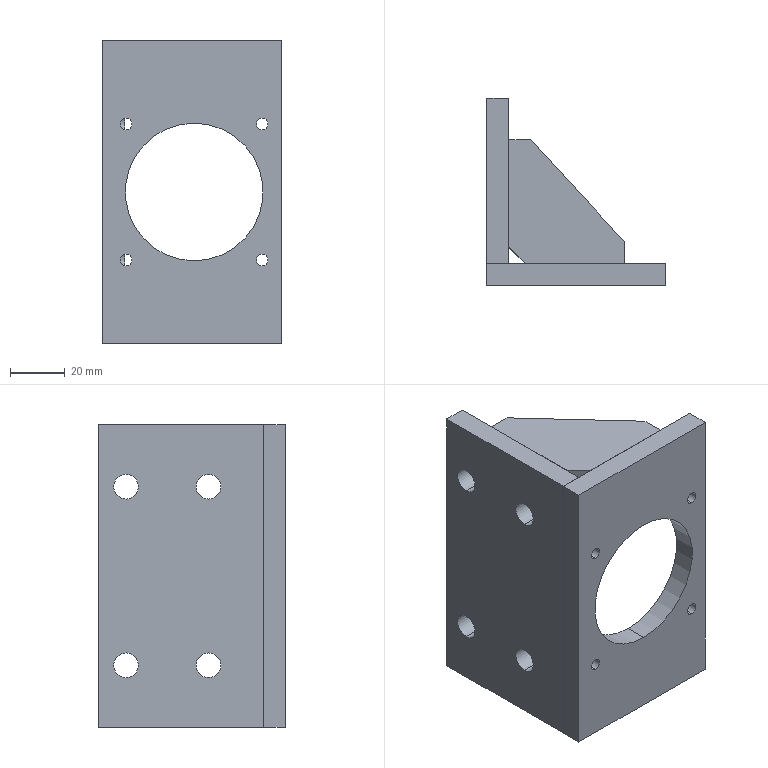Part | STEP file | Motor bracket | 4 solids | 50 faces | box 65 x 68 x 110 mm | volume 111617 mm3 | plane 28 | cylinder 20 | cone 2 | commonest cylinder face diameters 4.2 x10 9 x8 50.1 x2
STEP:
#1=CARTESIAN_POINT('',(-24.5,53.,55.));
#2=VERTEX_POINT('',#1);
#3=CARTESIAN_POINT('',(-24.5,14.,55.));
#4=VERTEX_POINT('',#3);
#5=CARTESIAN_POINT('',(-24.5,14.,55.));
#6=DIRECTION('',(0.,-1.,0.));
#7=VECTOR('',#6,1000.);
#8=LINE('',#5,#7);
#9=EDGE_CURVE('',#2,#4,#8,.T.);
#10=ORIENTED_EDGE('',*,*,#9,.F.);
#11=CARTESIAN_POINT('',(-24.5,53.,47.));
#12=VERTEX_POINT('',#11);
#13=CARTESIAN_POINT('',(-24.5,53.,47.));
#14=DIRECTION('',(0.,0.,1.));
#15=VECTOR('',#14,1000.);
#16=LINE('',#13,#15);
#17=EDGE_CURVE('',#12,#2,#16,.T.);
#18=ORIENTED_EDGE('',*,*,#17,.F.);
#19=CARTESIAN_POINT('',(-24.5,14.,47.));
#20=VERTEX_POINT('',#19);
#21=CARTESIAN_POINT('',(-24.5,14.,47.));
#22=DIRECTION('',(0.,-1.,0.));
#23=VECTOR('',#22,1000.);
#24=LINE('',#21,#23);
#25=EDGE_CURVE('',#12,#20,#24,.T.);
#26=ORIENTED_EDGE('',*,*,#25,.T.);
#27=CARTESIAN_POINT('',(-24.5,14.,47.));
#28=DIRECTION('',(0.,0.,1.));
#29=VECTOR('',#28,1000.);
#30=LINE('',#27,#29);
#31=EDGE_CURVE('',#20,#4,#30,.T.);
#32=ORIENTED_EDGE('',*,*,#31,.T.);
#33=EDGE_LOOP('',(#10,#18,#26,#32));
#34=FACE_OUTER_BOUND('',#33,.T.);
#35=CARTESIAN_POINT('',(-24.5,14.,47.));
#36=DIRECTION('',(-1.,0.,0.));
#37=DIRECTION('',(0.,0.,1.));
#38=AXIS2_PLACEMENT_3D('',#35,#36,#37);
#39=PLANE('',#38);
#40=ADVANCED_FACE('',(#34),#39,.T.);
#41=CARTESIAN_POINT('',(-16.5,53.,55.));
#42=VERTEX_POINT('',#41);
#43=CARTESIAN_POINT('',(-24.5,53.,55.));
#44=DIRECTION('',(-1.,0.,0.));
#45=VECTOR('',#44,1000.);
#46=LINE('',#43,#45);
#47=EDGE_CURVE('',#42,#2,#46,.T.);
#48=ORIENTED_EDGE('',*,*,#47,.F.);
#49=CARTESIAN_POINT('',(-16.5,53.,47.));
#50=VERTEX_POINT('',#49);
#51=CARTESIAN_POINT('',(-16.5,53.,47.));
#52=DIRECTION('',(0.,0.,1.));
#53=VECTOR('',#52,1000.);
#54=LINE('',#51,#53);
#55=EDGE_CURVE('',#50,#42,#54,.T.);
#56=ORIENTED_EDGE('',*,*,#55,.F.);
#57=CARTESIAN_POINT('',(-24.5,53.,47.));
#58=DIRECTION('',(-1.,0.,0.));
#59=VECTOR('',#58,1000.);
#60=LINE('',#57,#59);
#61=EDGE_CURVE('',#50,#12,#60,.T.);
#62=ORIENTED_EDGE('',*,*,#61,.T.);
#63=ORIENTED_EDGE('',*,*,#17,.T.);
#64=EDGE_LOOP('',(#48,#56,#62,#63));
#65=FACE_OUTER_BOUND('',#64,.T.);
#66=CARTESIAN_POINT('',(-24.5,53.,47.));
#67=DIRECTION('',(0.,1.,0.));
#68=DIRECTION('',(-1.,0.,0.));
#69=AXIS2_PLACEMENT_3D('',#66,#67,#68);
#70=PLANE('',#69);
#71=ADVANCED_FACE('',(#65),#70,.T.);
#72=CARTESIAN_POINT('',(17.5,16.,55.));
#73=VERTEX_POINT('',#72);
#74=CARTESIAN_POINT('',(-16.5,53.,55.));
#75=DIRECTION('',(-0.6766,0.7363,0.));
#76=VECTOR('',#75,1000.);
#77=LINE('',#74,#76);
#78=EDGE_CURVE('',#73,#42,#77,.T.);
#79=ORIENTED_EDGE('',*,*,#78,.F.);
#80=CARTESIAN_POINT('',(17.5,16.,47.));
#81=VERTEX_POINT('',#80);
#82=CARTESIAN_POINT('',(17.5,16.,47.));
#83=DIRECTION('',(0.,0.,1.));
#84=VECTOR('',#83,1000.);
#85=LINE('',#82,#84);
#86=EDGE_CURVE('',#81,#73,#85,.T.);
#87=ORIENTED_EDGE('',*,*,#86,.F.);
#88=CARTESIAN_POINT('',(-16.5,53.,47.));
#89=DIRECTION('',(-0.6766,0.7363,0.));
#90=VECTOR('',#89,1000.);
#91=LINE('',#88,#90);
#92=EDGE_CURVE('',#81,#50,#91,.T.);
#93=ORIENTED_EDGE('',*,*,#92,.T.);
#94=ORIENTED_EDGE('',*,*,#55,.T.);
#95=EDGE_LOOP('',(#79,#87,#93,#94));
#96=FACE_OUTER_BOUND('',#95,.T.);
#97=CARTESIAN_POINT('',(-16.5,53.,47.));
#98=DIRECTION('',(0.7363,0.6766,0.));
#99=DIRECTION('',(-0.6766,0.7363,0.));
#100=AXIS2_PLACEMENT_3D('',#97,#98,#99);
#101=PLANE('',#100);
#102=ADVANCED_FACE('',(#96),#101,.T.);
#103=CARTESIAN_POINT('',(17.5,8.,55.));
#104=VERTEX_POINT('',#103);
#105=CARTESIAN_POINT('',(17.5,16.,55.));
#106=DIRECTION('',(0.,1.,0.));
#107=VECTOR('',#106,1000.);
#108=LINE('',#105,#107);
#109=EDGE_CURVE('',#104,#73,#108,.T.);
#110=ORIENTED_EDGE('',*,*,#109,.F.);
#111=CARTESIAN_POINT('',(17.5,8.,47.));
#112=VERTEX_POINT('',#111);
#113=CARTESIAN_POINT('',(17.5,8.,47.));
#114=DIRECTION('',(0.,0.,1.));
#115=VECTOR('',#114,1000.);
#116=LINE('',#113,#115);
#117=EDGE_CURVE('',#112,#104,#116,.T.);
#118=ORIENTED_EDGE('',*,*,#117,.F.);
#119=CARTESIAN_POINT('',(17.5,16.,47.));
#120=DIRECTION('',(0.,1.,0.));
#121=VECTOR('',#120,1000.);
#122=LINE('',#119,#121);
#123=EDGE_CURVE('',#112,#81,#122,.T.);
#124=ORIENTED_EDGE('',*,*,#123,.T.);
#125=ORIENTED_EDGE('',*,*,#86,.T.);
#126=EDGE_LOOP('',(#110,#118,#124,#125));
#127=FACE_OUTER_BOUND('',#126,.T.);
#128=CARTESIAN_POINT('',(17.5,16.,47.));
#129=DIRECTION('',(1.,0.,0.));
#130=DIRECTION('',(0.,0.,-1.));
#131=AXIS2_PLACEMENT_3D('',#128,#129,#130);
#132=PLANE('',#131);
#133=ADVANCED_FACE('',(#127),#132,.T.);
#134=CARTESIAN_POINT('',(-18.5,8.,55.));
#135=VERTEX_POINT('',#134);
#136=CARTESIAN_POINT('',(17.5,8.,55.));
#137=DIRECTION('',(1.,0.,0.));
#138=VECTOR('',#137,1000.);
#139=LINE('',#136,#138);
#140=EDGE_CURVE('',#135,#104,#139,.T.);
#141=ORIENTED_EDGE('',*,*,#140,.F.);
#142=CARTESIAN_POINT('',(-18.5,8.,47.));
#143=VERTEX_POINT('',#142);
#144=CARTESIAN_POINT('',(-18.5,8.,47.));
#145=DIRECTION('',(0.,0.,1.));
#146=VECTOR('',#145,1000.);
#147=LINE('',#144,#146);
#148=EDGE_CURVE('',#143,#135,#147,.T.);
#149=ORIENTED_EDGE('',*,*,#148,.F.);
#150=CARTESIAN_POINT('',(17.5,8.,47.));
#151=DIRECTION('',(1.,0.,0.));
#152=VECTOR('',#151,1000.);
#153=LINE('',#150,#152);
#154=EDGE_CURVE('',#143,#112,#153,.T.);
#155=ORIENTED_EDGE('',*,*,#154,.T.);
#156=ORIENTED_EDGE('',*,*,#117,.T.);
#157=EDGE_LOOP('',(#141,#149,#155,#156));
#158=FACE_OUTER_BOUND('',#157,.T.);
#159=CARTESIAN_POINT('',(17.5,8.,47.));
#160=DIRECTION('',(0.,-1.,0.));
#161=DIRECTION('',(1.,0.,0.));
#162=AXIS2_PLACEMENT_3D('',#159,#160,#161);
#163=PLANE('',#162);
#164=ADVANCED_FACE('',(#158),#163,.T.);
#165=CARTESIAN_POINT('',(-18.5,8.,55.));
#166=DIRECTION('',(0.7071,-0.7071,0.));
#167=VECTOR('',#166,1000.);
#168=LINE('',#165,#167);
#169=EDGE_CURVE('',#4,#135,#168,.T.);
#170=ORIENTED_EDGE('',*,*,#169,.F.);
#171=ORIENTED_EDGE('',*,*,#31,.F.);
#172=CARTESIAN_POINT('',(-18.5,8.,47.));
#173=DIRECTION('',(0.7071,-0.7071,0.));
#174=VECTOR('',#173,1000.);
#175=LINE('',#172,#174);
#176=EDGE_CURVE('',#20,#143,#175,.T.);
#177=ORIENTED_EDGE('',*,*,#176,.T.);
#178=ORIENTED_EDGE('',*,*,#148,.T.);
#179=EDGE_LOOP('',(#170,#171,#177,#178));
#180=FACE_OUTER_BOUND('',#179,.T.);
#181=CARTESIAN_POINT('',(-18.5,8.,47.));
#182=DIRECTION('',(-0.7071,-0.7071,0.));
#183=DIRECTION('',(0.7071,-0.7071,0.));
#184=AXIS2_PLACEMENT_3D('',#181,#182,#183);
#185=PLANE('',#184);
#186=ADVANCED_FACE('',(#180),#185,.T.);
#187=ORIENTED_EDGE('',*,*,#25,.F.);
#188=ORIENTED_EDGE('',*,*,#61,.F.);
#189=ORIENTED_EDGE('',*,*,#92,.F.);
#190=ORIENTED_EDGE('',*,*,#123,.F.);
#191=ORIENTED_EDGE('',*,*,#154,.F.);
#192=ORIENTED_EDGE('',*,*,#176,.F.);
#193=EDGE_LOOP('',(#187,#188,#189,#190,#191,#192));
#194=FACE_OUTER_BOUND('',#193,.T.);
#195=CARTESIAN_POINT('',(0.,0.,47.));
#196=DIRECTION('',(0.,0.,-1.));
#197=DIRECTION('',(-1.,0.,0.));
#198=AXIS2_PLACEMENT_3D('',#195,#196,#197);
#199=PLANE('',#198);
#200=ADVANCED_FACE('',(#194),#199,.T.);
#201=ORIENTED_EDGE('',*,*,#9,.T.);
#202=ORIENTED_EDGE('',*,*,#169,.T.);
#203=ORIENTED_EDGE('',*,*,#140,.T.);
#204=ORIENTED_EDGE('',*,*,#109,.T.);
#205=ORIENTED_EDGE('',*,*,#78,.T.);
#206=ORIENTED_EDGE('',*,*,#47,.T.);
#207=EDGE_LOOP('',(#201,#202,#203,#204,#205,#206));
#208=FACE_OUTER_BOUND('',#207,.T.);
#209=CARTESIAN_POINT('',(0.,0.,55.));
#210=DIRECTION('',(0.,0.,-1.));
#211=DIRECTION('',(-1.,0.,0.));
#212=AXIS2_PLACEMENT_3D('',#209,#210,#211);
#213=PLANE('',#212);
#214=ADVANCED_FACE('',(#208),#213,.F.);
#215=CLOSED_SHELL('',(#40,#71,#102,#133,#164,#186,#200,#214));
#216=MANIFOLD_SOLID_BREP('',#215);
#217=CARTESIAN_POINT('',(-24.5,53.,-55.));
#218=VERTEX_POINT('',#217);
#219=CARTESIAN_POINT('',(-24.5,14.,-55.));
#220=VERTEX_POINT('',#219);
#221=CARTESIAN_POINT('',(-24.5,14.,-55.));
#222=DIRECTION('',(0.,-1.,0.));
#223=VECTOR('',#222,1000.);
#224=LINE('',#221,#223);
#225=EDGE_CURVE('',#218,#220,#224,.T.);
#226=ORIENTED_EDGE('',*,*,#225,.T.);
#227=CARTESIAN_POINT('',(-24.5,14.,-47.));
#228=VERTEX_POINT('',#227);
#229=CARTESIAN_POINT('',(-24.5,14.,-47.));
#230=DIRECTION('',(0.,0.,-1.));
#231=VECTOR('',#230,1000.);
#232=LINE('',#229,#231);
#233=EDGE_CURVE('',#228,#220,#232,.T.);
#234=ORIENTED_EDGE('',*,*,#233,.F.);
#235=CARTESIAN_POINT('',(-24.5,53.,-47.));
#236=VERTEX_POINT('',#235);
#237=CARTESIAN_POINT('',(-24.5,14.,-47.));
#238=DIRECTION('',(0.,-1.,0.));
#239=VECTOR('',#238,1000.);
#240=LINE('',#237,#239);
#241=EDGE_CURVE('',#236,#228,#240,.T.);
#242=ORIENTED_EDGE('',*,*,#241,.F.);
#243=CARTESIAN_POINT('',(-24.5,53.,-47.));
#244=DIRECTION('',(0.,0.,-1.));
#245=VECTOR('',#244,1000.);
#246=LINE('',#243,#245);
#247=EDGE_CURVE('',#236,#218,#246,.T.);
#248=ORIENTED_EDGE('',*,*,#247,.T.);
#249=EDGE_LOOP('',(#226,#234,#242,#248));
#250=FACE_OUTER_BOUND('',#249,.T.);
#251=CARTESIAN_POINT('',(-24.5,14.,-47.));
#252=DIRECTION('',(-1.,0.,0.));
#253=DIRECTION('',(0.,0.,-1.));
#254=AXIS2_PLACEMENT_3D('',#251,#252,#253);
#255=PLANE('',#254);
#256=ADVANCED_FACE('',(#250),#255,.T.);
#257=CARTESIAN_POINT('',(-16.5,53.,-55.));
#258=VERTEX_POINT('',#257);
#259=CARTESIAN_POINT('',(-24.5,53.,-55.));
#260=DIRECTION('',(-1.,0.,0.));
#261=VECTOR('',#260,1000.);
#262=LINE('',#259,#261);
#263=EDGE_CURVE('',#258,#218,#262,.T.);
#264=ORIENTED_EDGE('',*,*,#263,.T.);
#265=ORIENTED_EDGE('',*,*,#247,.F.);
#266=CARTESIAN_POINT('',(-16.5,53.,-47.));
#267=VERTEX_POINT('',#266);
#268=CARTESIAN_POINT('',(-24.5,53.,-47.));
#269=DIRECTION('',(-1.,0.,0.));
#270=VECTOR('',#269,1000.);
#271=LINE('',#268,#270);
#272=EDGE_CURVE('',#267,#236,#271,.T.);
#273=ORIENTED_EDGE('',*,*,#272,.F.);
#274=CARTESIAN_POINT('',(-16.5,53.,-47.));
#275=DIRECTION('',(0.,0.,-1.));
#276=VECTOR('',#275,1000.);
#277=LINE('',#274,#276);
#278=EDGE_CURVE('',#267,#258,#277,.T.);
#279=ORIENTED_EDGE('',*,*,#278,.T.);
#280=EDGE_LOOP('',(#264,#265,#273,#279));
#281=FACE_OUTER_BOUND('',#280,.T.);
#282=CARTESIAN_POINT('',(-24.5,53.,-47.));
#283=DIRECTION('',(0.,1.,0.));
#284=DIRECTION('',(-1.,0.,0.));
#285=AXIS2_PLACEMENT_3D('',#282,#283,#284);
#286=PLANE('',#285);
#287=ADVANCED_FACE('',(#281),#286,.T.);
#288=CARTESIAN_POINT('',(17.5,16.,-55.));
#289=VERTEX_POINT('',#288);
#290=CARTESIAN_POINT('',(-16.5,53.,-55.));
#291=DIRECTION('',(-0.6766,0.7363,0.));
#292=VECTOR('',#291,1000.);
#293=LINE('',#290,#292);
#294=EDGE_CURVE('',#289,#258,#293,.T.);
#295=ORIENTED_EDGE('',*,*,#294,.T.);
#296=ORIENTED_EDGE('',*,*,#278,.F.);
#297=CARTESIAN_POINT('',(17.5,16.,-47.));
#298=VERTEX_POINT('',#297);
#299=CARTESIAN_POINT('',(-16.5,53.,-47.));
#300=DIRECTION('',(-0.6766,0.7363,0.));
#301=VECTOR('',#300,1000.);
#302=LINE('',#299,#301);
#303=EDGE_CURVE('',#298,#267,#302,.T.);
#304=ORIENTED_EDGE('',*,*,#303,.F.);
#305=CARTESIAN_POINT('',(17.5,16.,-47.));
#306=DIRECTION('',(0.,0.,-1.));
#307=VECTOR('',#306,1000.);
#308=LINE('',#305,#307);
#309=EDGE_CURVE('',#298,#289,#308,.T.);
#310=ORIENTED_EDGE('',*,*,#309,.T.);
#311=EDGE_LOOP('',(#295,#296,#304,#310));
#312=FACE_OUTER_BOUND('',#311,.T.);
#313=CARTESIAN_POINT('',(-16.5,53.,-47.));
#314=DIRECTION('',(0.7363,0.6766,0.));
#315=DIRECTION('',(-0.6766,0.7363,0.));
#316=AXIS2_PLACEMENT_3D('',#313,#314,#315);
#317=PLANE('',#316);
#318=ADVANCED_FACE('',(#312),#317,.T.);
#319=CARTESIAN_POINT('',(17.5,8.,-55.));
#320=VERTEX_POINT('',#319);
#321=CARTESIAN_POINT('',(17.5,16.,-55.));
#322=DIRECTION('',(0.,1.,0.));
#323=VECTOR('',#322,1000.);
#324=LINE('',#321,#323);
#325=EDGE_CURVE('',#320,#289,#324,.T.);
#326=ORIENTED_EDGE('',*,*,#325,.T.);
#327=ORIENTED_EDGE('',*,*,#309,.F.);
#328=CARTESIAN_POINT('',(17.5,8.,-47.));
#329=VERTEX_POINT('',#328);
#330=CARTESIAN_POINT('',(17.5,16.,-47.));
#331=DIRECTION('',(0.,1.,0.));
#332=VECTOR('',#331,1000.);
#333=LINE('',#330,#332);
#334=EDGE_CURVE('',#329,#298,#333,.T.);
#335=ORIENTED_EDGE('',*,*,#334,.F.);
#336=CARTESIAN_POINT('',(17.5,8.,-47.));
#337=DIRECTION('',(0.,0.,-1.));
#338=VECTOR('',#337,1000.);
#339=LINE('',#336,#338);
#340=EDGE_CURVE('',#329,#320,#339,.T.);
#341=ORIENTED_EDGE('',*,*,#340,.T.);
#342=EDGE_LOOP('',(#326,#327,#335,#341));
#343=FACE_OUTER_BOUND('',#342,.T.);
#344=CARTESIAN_POINT('',(17.5,16.,-47.));
#345=DIRECTION('',(1.,0.,0.));
#346=DIRECTION('',(0.,0.,1.));
#347=AXIS2_PLACEMENT_3D('',#344,#345,#346);
#348=PLANE('',#347);
#349=ADVANCED_FACE('',(#343),#348,.T.);
#350=CARTESIAN_POINT('',(-18.5,8.,-55.));
#351=VERTEX_POINT('',#350);
#352=CARTESIAN_POINT('',(17.5,8.,-55.));
#353=DIRECTION('',(1.,0.,0.));
#354=VECTOR('',#353,1000.);
#355=LINE('',#352,#354);
#356=EDGE_CURVE('',#351,#320,#355,.T.);
#357=ORIENTED_EDGE('',*,*,#356,.T.);
#358=ORIENTED_EDGE('',*,*,#340,.F.);
#359=CARTESIAN_POINT('',(-18.5,8.,-47.));
#360=VERTEX_POINT('',#359);
#361=CARTESIAN_POINT('',(17.5,8.,-47.));
#362=DIRECTION('',(1.,0.,0.));
#363=VECTOR('',#362,1000.);
#364=LINE('',#361,#363);
#365=EDGE_CURVE('',#360,#329,#364,.T.);
#366=ORIENTED_EDGE('',*,*,#365,.F.);
#367=CARTESIAN_POINT('',(-18.5,8.,-47.));
#368=DIRECTION('',(0.,0.,-1.));
#369=VECTOR('',#368,1000.);
#370=LINE('',#367,#369);
#371=EDGE_CURVE('',#360,#351,#370,.T.);
#372=ORIENTED_EDGE('',*,*,#371,.T.);
#373=EDGE_LOOP('',(#357,#358,#366,#372));
#374=FACE_OUTER_BOUND('',#373,.T.);
#375=CARTESIAN_POINT('',(17.5,8.,-47.));
#376=DIRECTION('',(0.,-1.,0.));
#377=DIRECTION('',(1.,0.,0.));
#378=AXIS2_PLACEMENT_3D('',#375,#376,#377);
#379=PLANE('',#378);
#380=ADVANCED_FACE('',(#374),#379,.T.);
#381=CARTESIAN_POINT('',(-18.5,8.,-55.));
#382=DIRECTION('',(0.7071,-0.7071,0.));
#383=VECTOR('',#382,1000.);
#384=LINE('',#381,#383);
#385=EDGE_CURVE('',#220,#351,#384,.T.);
#386=ORIENTED_EDGE('',*,*,#385,.T.);
#387=ORIENTED_EDGE('',*,*,#371,.F.);
#388=CARTESIAN_POINT('',(-18.5,8.,-47.));
#389=DIRECTION('',(0.7071,-0.7071,0.));
#390=VECTOR('',#389,1000.);
#391=LINE('',#388,#390);
#392=EDGE_CURVE('',#228,#360,#391,.T.);
#393=ORIENTED_EDGE('',*,*,#392,.F.);
#394=ORIENTED_EDGE('',*,*,#233,.T.);
#395=EDGE_LOOP('',(#386,#387,#393,#394));
#396=FACE_OUTER_BOUND('',#395,.T.);
#397=CARTESIAN_POINT('',(-18.5,8.,-47.));
#398=DIRECTION('',(-0.7071,-0.7071,0.));
#399=DIRECTION('',(0.7071,-0.7071,0.));
#400=AXIS2_PLACEMENT_3D('',#397,#398,#399);
#401=PLANE('',#400);
#402=ADVANCED_FACE('',(#396),#401,.T.);
#403=ORIENTED_EDGE('',*,*,#241,.T.);
#404=ORIENTED_EDGE('',*,*,#392,.T.);
#405=ORIENTED_EDGE('',*,*,#365,.T.);
#406=ORIENTED_EDGE('',*,*,#334,.T.);
#407=ORIENTED_EDGE('',*,*,#303,.T.);
#408=ORIENTED_EDGE('',*,*,#272,.T.);
#409=EDGE_LOOP('',(#403,#404,#405,#406,#407,#408));
#410=FACE_OUTER_BOUND('',#409,.T.);
#411=CARTESIAN_POINT('',(0.,0.,-47.));
#412=DIRECTION('',(0.,0.,1.));
#413=DIRECTION('',(-1.,0.,0.));
#414=AXIS2_PLACEMENT_3D('',#411,#412,#413);
#415=PLANE('',#414);
#416=ADVANCED_FACE('',(#410),#415,.T.);
#417=ORIENTED_EDGE('',*,*,#225,.F.);
#418=ORIENTED_EDGE('',*,*,#263,.F.);
#419=ORIENTED_EDGE('',*,*,#294,.F.);
#420=ORIENTED_EDGE('',*,*,#325,.F.);
#421=ORIENTED_EDGE('',*,*,#356,.F.);
#422=ORIENTED_EDGE('',*,*,#385,.F.);
#423=EDGE_LOOP('',(#417,#418,#419,#420,#421,#422));
#424=FACE_OUTER_BOUND('',#423,.T.);
#425=CARTESIAN_POINT('',(0.,0.,-55.));
#426=DIRECTION('',(0.,0.,1.));
#427=DIRECTION('',(-1.,0.,0.));
#428=AXIS2_PLACEMENT_3D('',#425,#426,#427);
#429=PLANE('',#428);
#430=ADVANCED_FACE('',(#424),#429,.F.);
#431=CLOSED_SHELL('',(#256,#287,#318,#349,#380,#402,#416,#430));
#432=MANIFOLD_SOLID_BREP('',#431);
#433=CARTESIAN_POINT('',(-32.5,28.,28.));
#434=VERTEX_POINT('',#433);
#435=CARTESIAN_POINT('',(-32.5,28.,37.));
#436=VERTEX_POINT('',#435);
#437=CARTESIAN_POINT('',(-32.5,28.,32.5));
#438=DIRECTION('',(-1.,0.,0.));
#439=DIRECTION('',(0.,0.,1.));
#440=AXIS2_PLACEMENT_3D('',#437,#438,#439);
#441=CIRCLE('',#440,4.5);
#442=EDGE_CURVE('',#434,#436,#441,.T.);
#443=ORIENTED_EDGE('',*,*,#442,.T.);
#444=CARTESIAN_POINT('',(-24.5,28.,37.));
#445=VERTEX_POINT('',#444);
#446=CARTESIAN_POINT('',(-24.5,28.,37.));
#447=DIRECTION('',(1.,0.,0.));
#448=VECTOR('',#447,1000.);
#449=LINE('',#446,#448);
#450=EDGE_CURVE('',#436,#445,#449,.T.);
#451=ORIENTED_EDGE('',*,*,#450,.T.);
#452=CARTESIAN_POINT('',(-24.5,28.,28.));
#453=VERTEX_POINT('',#452);
#454=CARTESIAN_POINT('',(-24.5,28.,32.5));
#455=DIRECTION('',(1.,0.,0.));
#456=DIRECTION('',(0.,0.,-1.));
#457=AXIS2_PLACEMENT_3D('',#454,#455,#456);
#458=CIRCLE('',#457,4.5);
#459=EDGE_CURVE('',#445,#453,#458,.T.);
#460=ORIENTED_EDGE('',*,*,#459,.T.);
#461=CARTESIAN_POINT('',(-24.5,28.,28.));
#462=DIRECTION('',(1.,0.,0.));
#463=VECTOR('',#462,1000.);
#464=LINE('',#461,#463);
#465=EDGE_CURVE('',#434,#453,#464,.T.);
#466=ORIENTED_EDGE('',*,*,#465,.F.);
#467=EDGE_LOOP('',(#443,#451,#460,#466));
#468=FACE_OUTER_BOUND('',#467,.T.);
#469=CARTESIAN_POINT('',(-24.5,28.,32.5));
#470=DIRECTION('',(1.,0.,0.));
#471=DIRECTION('',(0.,0.,-1.));
#472=AXIS2_PLACEMENT_3D('',#469,#470,#471);
#473=CYLINDRICAL_SURFACE('',#472,4.5);
#474=ADVANCED_FACE('',(#468),#473,.F.);
#475=CARTESIAN_POINT('',(-32.5,58.,28.));
#476=VERTEX_POINT('',#475);
#477=CARTESIAN_POINT('',(-32.5,58.,37.));
#478=VERTEX_POINT('',#477);
#479=CARTESIAN_POINT('',(-32.5,58.,32.5));
#480=DIRECTION('',(-1.,0.,0.));
#481=DIRECTION('',(0.,0.,1.));
#482=AXIS2_PLACEMENT_3D('',#479,#480,#481);
#483=CIRCLE('',#482,4.5);
#484=EDGE_CURVE('',#476,#478,#483,.T.);
#485=ORIENTED_EDGE('',*,*,#484,.T.);
#486=CARTESIAN_POINT('',(-24.5,58.,37.));
#487=VERTEX_POINT('',#486);
#488=CARTESIAN_POINT('',(-24.5,58.,37.));
#489=DIRECTION('',(1.,0.,0.));
#490=VECTOR('',#489,1000.);
#491=LINE('',#488,#490);
#492=EDGE_CURVE('',#478,#487,#491,.T.);
#493=ORIENTED_EDGE('',*,*,#492,.T.);
#494=CARTESIAN_POINT('',(-24.5,58.,28.));
#495=VERTEX_POINT('',#494);
#496=CARTESIAN_POINT('',(-24.5,58.,32.5));
#497=DIRECTION('',(1.,0.,0.));
#498=DIRECTION('',(0.,0.,-1.));
#499=AXIS2_PLACEMENT_3D('',#496,#497,#498);
#500=CIRCLE('',#499,4.5);
#501=EDGE_CURVE('',#487,#495,#500,.T.);
#502=ORIENTED_EDGE('',*,*,#501,.T.);
#503=CARTESIAN_POINT('',(-24.5,58.,28.));
#504=DIRECTION('',(1.,0.,0.));
#505=VECTOR('',#504,1000.);
#506=LINE('',#503,#505);
#507=EDGE_CURVE('',#476,#495,#506,.T.);
#508=ORIENTED_EDGE('',*,*,#507,.F.);
#509=EDGE_LOOP('',(#485,#493,#502,#508));
#510=FACE_OUTER_BOUND('',#509,.T.);
#511=CARTESIAN_POINT('',(-24.5,58.,32.5));
#512=DIRECTION('',(1.,0.,0.));
#513=DIRECTION('',(0.,0.,-1.));
#514=AXIS2_PLACEMENT_3D('',#511,#512,#513);
#515=CYLINDRICAL_SURFACE('',#514,4.5);
#516=ADVANCED_FACE('',(#510),#515,.F.);
#517=CARTESIAN_POINT('',(-32.5,28.,-37.));
#518=VERTEX_POINT('',#517);
#519=CARTESIAN_POINT('',(-32.5,28.,-28.));
#520=VERTEX_POINT('',#519);
#521=CARTESIAN_POINT('',(-32.5,28.,-32.5));
#522=DIRECTION('',(-1.,0.,0.));
#523=DIRECTION('',(0.,0.,1.));
#524=AXIS2_PLACEMENT_3D('',#521,#522,#523);
#525=CIRCLE('',#524,4.5);
#526=EDGE_CURVE('',#518,#520,#525,.T.);
#527=ORIENTED_EDGE('',*,*,#526,.T.);
#528=CARTESIAN_POINT('',(-24.5,28.,-28.));
#529=VERTEX_POINT('',#528);
#530=CARTESIAN_POINT('',(-24.5,28.,-28.));
#531=DIRECTION('',(1.,0.,0.));
#532=VECTOR('',#531,1000.);
#533=LINE('',#530,#532);
#534=EDGE_CURVE('',#520,#529,#533,.T.);
#535=ORIENTED_EDGE('',*,*,#534,.T.);
#536=CARTESIAN_POINT('',(-24.5,28.,-37.));
#537=VERTEX_POINT('',#536);
#538=CARTESIAN_POINT('',(-24.5,28.,-32.5));
#539=DIRECTION('',(1.,0.,0.));
#540=DIRECTION('',(0.,0.,-1.));
#541=AXIS2_PLACEMENT_3D('',#538,#539,#540);
#542=CIRCLE('',#541,4.5);
#543=EDGE_CURVE('',#529,#537,#542,.T.);
#544=ORIENTED_EDGE('',*,*,#543,.T.);
#545=CARTESIAN_POINT('',(-24.5,28.,-37.));
#546=DIRECTION('',(1.,0.,0.));
#547=VECTOR('',#546,1000.);
#548=LINE('',#545,#547);
#549=EDGE_CURVE('',#518,#537,#548,.T.);
#550=ORIENTED_EDGE('',*,*,#549,.F.);
#551=EDGE_LOOP('',(#527,#535,#544,#550));
#552=FACE_OUTER_BOUND('',#551,.T.);
#553=CARTESIAN_POINT('',(-24.5,28.,-32.5));
#554=DIRECTION('',(1.,0.,0.));
#555=DIRECTION('',(0.,0.,-1.));
#556=AXIS2_PLACEMENT_3D('',#553,#554,#555);
#557=CYLINDRICAL_SURFACE('',#556,4.5);
#558=ADVANCED_FACE('',(#552),#557,.F.);
#559=CARTESIAN_POINT('',(-32.5,58.,-37.));
#560=VERTEX_POINT('',#559);
#561=CARTESIAN_POINT('',(-32.5,58.,-28.));
#562=VERTEX_POINT('',#561);
#563=CARTESIAN_POINT('',(-32.5,58.,-32.5));
#564=DIRECTION('',(-1.,0.,0.));
#565=DIRECTION('',(0.,0.,1.));
#566=AXIS2_PLACEMENT_3D('',#563,#564,#565);
#567=CIRCLE('',#566,4.5);
#568=EDGE_CURVE('',#560,#562,#567,.T.);
#569=ORIENTED_EDGE('',*,*,#568,.T.);
#570=CARTESIAN_POINT('',(-24.5,58.,-28.));
#571=VERTEX_POINT('',#570);
#572=CARTESIAN_POINT('',(-24.5,58.,-28.));
#573=DIRECTION('',(1.,0.,0.));
#574=VECTOR('',#573,1000.);
#575=LINE('',#572,#574);
#576=EDGE_CURVE('',#562,#571,#575,.T.);
#577=ORIENTED_EDGE('',*,*,#576,.T.);
#578=CARTESIAN_POINT('',(-24.5,58.,-37.));
#579=VERTEX_POINT('',#578);
#580=CARTESIAN_POINT('',(-24.5,58.,-32.5));
#581=DIRECTION('',(1.,0.,0.));
#582=DIRECTION('',(0.,0.,-1.));
#583=AXIS2_PLACEMENT_3D('',#580,#581,#582);
#584=CIRCLE('',#583,4.5);
#585=EDGE_CURVE('',#571,#579,#584,.T.);
#586=ORIENTED_EDGE('',*,*,#585,.T.);
#587=CARTESIAN_POINT('',(-24.5,58.,-37.));
#588=DIRECTION('',(1.,0.,0.));
#589=VECTOR('',#588,1000.);
#590=LINE('',#587,#589);
#591=EDGE_CURVE('',#560,#579,#590,.T.);
#592=ORIENTED_EDGE('',*,*,#591,.F.);
#593=EDGE_LOOP('',(#569,#577,#586,#592));
#594=FACE_OUTER_BOUND('',#593,.T.);
#595=CARTESIAN_POINT('',(-24.5,58.,-32.5));
#596=DIRECTION('',(1.,0.,0.));
#597=DIRECTION('',(0.,0.,-1.));
#598=AXIS2_PLACEMENT_3D('',#595,#596,#597);
#599=CYLINDRICAL_SURFACE('',#598,4.5);
#600=ADVANCED_FACE('',(#594),#599,.F.);
#601=CARTESIAN_POINT('',(-32.5,68.,-55.));
#602=VERTEX_POINT('',#601);
#603=CARTESIAN_POINT('',(-32.5,8.,-55.));
#604=VERTEX_POINT('',#603);
#605=CARTESIAN_POINT('',(-32.5,68.,-55.));
#606=DIRECTION('',(0.,-1.,0.));
#607=VECTOR('',#606,1000.);
#608=LINE('',#605,#607);
#609=EDGE_CURVE('',#602,#604,#608,.T.);
#610=ORIENTED_EDGE('',*,*,#609,.F.);
#611=CARTESIAN_POINT('',(-24.5,68.,-55.));
#612=VERTEX_POINT('',#611);
#613=CARTESIAN_POINT('',(-24.5,68.,-55.));
#614=DIRECTION('',(-1.,0.,0.));
#615=VECTOR('',#614,1000.);
#616=LINE('',#613,#615);
#617=EDGE_CURVE('',#612,#602,#616,.T.);
#618=ORIENTED_EDGE('',*,*,#617,.F.);
#619=CARTESIAN_POINT('',(-24.5,8.,-55.));
#620=VERTEX_POINT('',#619);
#621=CARTESIAN_POINT('',(-24.5,68.,-55.));
#622=DIRECTION('',(0.,-1.,0.));
#623=VECTOR('',#622,1000.);
#624=LINE('',#621,#623);
#625=EDGE_CURVE('',#612,#620,#624,.T.);
#626=ORIENTED_EDGE('',*,*,#625,.T.);
#627=CARTESIAN_POINT('',(-24.5,8.,-55.));
#628=DIRECTION('',(-1.,0.,0.));
#629=VECTOR('',#628,1000.);
#630=LINE('',#627,#629);
#631=EDGE_CURVE('',#620,#604,#630,.T.);
#632=ORIENTED_EDGE('',*,*,#631,.T.);
#633=EDGE_LOOP('',(#610,#618,#626,#632));
#634=FACE_OUTER_BOUND('',#633,.T.);
#635=CARTESIAN_POINT('',(-24.5,68.,-55.));
#636=DIRECTION('',(0.,0.,-1.));
#637=DIRECTION('',(-1.,0.,0.));
#638=AXIS2_PLACEMENT_3D('',#635,#636,#637);
#639=PLANE('',#638);
#640=ADVANCED_FACE('',(#634),#639,.T.);
#641=CARTESIAN_POINT('',(-32.5,68.,55.));
#642=VERTEX_POINT('',#641);
#643=CARTESIAN_POINT('',(-32.5,68.,55.));
#644=DIRECTION('',(0.,0.,-1.));
#645=VECTOR('',#644,1000.);
#646=LINE('',#643,#645);
#647=EDGE_CURVE('',#642,#602,#646,.T.);
#648=ORIENTED_EDGE('',*,*,#647,.F.);
#649=CARTESIAN_POINT('',(-24.5,68.,55.));
#650=VERTEX_POINT('',#649);
#651=CARTESIAN_POINT('',(-24.5,68.,55.));
#652=DIRECTION('',(-1.,0.,0.));
#653=VECTOR('',#652,1000.);
#654=LINE('',#651,#653);
#655=EDGE_CURVE('',#650,#642,#654,.T.);
#656=ORIENTED_EDGE('',*,*,#655,.F.);
#657=CARTESIAN_POINT('',(-24.5,68.,55.));
#658=DIRECTION('',(0.,0.,-1.));
#659=VECTOR('',#658,1000.);
#660=LINE('',#657,#659);
#661=EDGE_CURVE('',#650,#612,#660,.T.);
#662=ORIENTED_EDGE('',*,*,#661,.T.);
#663=ORIENTED_EDGE('',*,*,#617,.T.);
#664=EDGE_LOOP('',(#648,#656,#662,#663));
#665=FACE_OUTER_BOUND('',#664,.T.);
#666=CARTESIAN_POINT('',(-24.5,68.,55.));
#667=DIRECTION('',(0.,1.,0.));
#668=DIRECTION('',(0.,0.,1.));
#669=AXIS2_PLACEMENT_3D('',#666,#667,#668);
#670=PLANE('',#669);
#671=ADVANCED_FACE('',(#665),#670,.T.);
#672=CARTESIAN_POINT('',(-32.5,8.,55.));
#673=VERTEX_POINT('',#672);
#674=CARTESIAN_POINT('',(-32.5,8.,55.));
#675=DIRECTION('',(0.,1.,0.));
#676=VECTOR('',#675,1000.);
#677=LINE('',#674,#676);
#678=EDGE_CURVE('',#673,#642,#677,.T.);
#679=ORIENTED_EDGE('',*,*,#678,.F.);
#680=CARTESIAN_POINT('',(-24.5,8.,55.));
#681=VERTEX_POINT('',#680);
#682=CARTESIAN_POINT('',(-24.5,8.,55.));
#683=DIRECTION('',(-1.,0.,0.));
#684=VECTOR('',#683,1000.);
#685=LINE('',#682,#684);
#686=EDGE_CURVE('',#681,#673,#685,.T.);
#687=ORIENTED_EDGE('',*,*,#686,.F.);
#688=CARTESIAN_POINT('',(-24.5,8.,55.));
#689=DIRECTION('',(0.,1.,0.));
#690=VECTOR('',#689,1000.);
#691=LINE('',#688,#690);
#692=EDGE_CURVE('',#681,#650,#691,.T.);
#693=ORIENTED_EDGE('',*,*,#692,.T.);
#694=ORIENTED_EDGE('',*,*,#655,.T.);
#695=EDGE_LOOP('',(#679,#687,#693,#694));
#696=FACE_OUTER_BOUND('',#695,.T.);
#697=CARTESIAN_POINT('',(-24.5,8.,55.));
#698=DIRECTION('',(0.,0.,1.));
#699=DIRECTION('',(1.,0.,0.));
#700=AXIS2_PLACEMENT_3D('',#697,#698,#699);
#701=PLANE('',#700);
#702=ADVANCED_FACE('',(#696),#701,.T.);
#703=CARTESIAN_POINT('',(-24.5,8.,26.775));
#704=VERTEX_POINT('',#703);
#705=CARTESIAN_POINT('',(-24.5,8.,22.722));
#706=VERTEX_POINT('',#705);
#707=CARTESIAN_POINT('',(-23.949,8.,24.749));
#708=DIRECTION('',(0.,-1.,0.));
#709=DIRECTION('',(0.,0.,-1.));
#710=AXIS2_PLACEMENT_3D('',#707,#708,#709);
#711=CIRCLE('',#710,2.1);
#712=EDGE_CURVE('',#704,#706,#711,.T.);
#713=ORIENTED_EDGE('',*,*,#712,.F.);
#714=CARTESIAN_POINT('',(-24.5,8.,-55.));
#715=DIRECTION('',(0.,0.,1.));
#716=VECTOR('',#715,1000.);
#717=LINE('',#714,#716);
#718=EDGE_CURVE('',#704,#681,#717,.T.);
#719=ORIENTED_EDGE('',*,*,#718,.T.);
#720=ORIENTED_EDGE('',*,*,#686,.T.);
#721=CARTESIAN_POINT('',(-32.5,8.,-55.));
#722=DIRECTION('',(0.,0.,1.));
#723=VECTOR('',#722,1000.);
#724=LINE('',#721,#723);
#725=EDGE_CURVE('',#604,#673,#724,.T.);
#726=ORIENTED_EDGE('',*,*,#725,.F.);
#727=ORIENTED_EDGE('',*,*,#631,.F.);
#728=CARTESIAN_POINT('',(-24.5,8.,-26.775));
#729=VERTEX_POINT('',#728);
#730=CARTESIAN_POINT('',(-24.5,8.,-55.));
#731=DIRECTION('',(0.,0.,1.));
#732=VECTOR('',#731,1000.);
#733=LINE('',#730,#732);
#734=EDGE_CURVE('',#620,#729,#733,.T.);
#735=ORIENTED_EDGE('',*,*,#734,.T.);
#736=CARTESIAN_POINT('',(-24.5,8.,-22.722));
#737=VERTEX_POINT('',#736);
#738=CARTESIAN_POINT('',(-23.949,8.,-24.749));
#739=DIRECTION('',(0.,-1.,0.));
#740=DIRECTION('',(0.,0.,-1.));
#741=AXIS2_PLACEMENT_3D('',#738,#739,#740);
#742=CIRCLE('',#741,2.1);
#743=EDGE_CURVE('',#737,#729,#742,.T.);
#744=ORIENTED_EDGE('',*,*,#743,.F.);
#745=CARTESIAN_POINT('',(-24.5,8.,-55.));
#746=DIRECTION('',(0.,0.,1.));
#747=VECTOR('',#746,1000.);
#748=LINE('',#745,#747);
#749=EDGE_CURVE('',#737,#706,#748,.T.);
#750=ORIENTED_EDGE('',*,*,#749,.T.);
#751=EDGE_LOOP('',(#713,#719,#720,#726,#727,#735,#744,#750));
#752=FACE_OUTER_BOUND('',#751,.T.);
#753=CARTESIAN_POINT('',(-24.5,8.,-55.));
#754=DIRECTION('',(0.,-1.,0.));
#755=DIRECTION('',(0.,0.,-1.));
#756=AXIS2_PLACEMENT_3D('',#753,#754,#755);
#757=PLANE('',#756);
#758=ADVANCED_FACE('',(#752),#757,.T.);
#759=CARTESIAN_POINT('',(-24.5,28.,32.5));
#760=DIRECTION('',(1.,0.,0.));
#761=DIRECTION('',(0.,0.,-1.));
#762=AXIS2_PLACEMENT_3D('',#759,#760,#761);
#763=CIRCLE('',#762,4.5);
#764=EDGE_CURVE('',#453,#445,#763,.T.);
#765=ORIENTED_EDGE('',*,*,#764,.F.);
#766=ORIENTED_EDGE('',*,*,#459,.F.);
#767=EDGE_LOOP('',(#765,#766));
#768=FACE_BOUND('',#767,.T.);
#769=CARTESIAN_POINT('',(-24.5,58.,32.5));
#770=DIRECTION('',(1.,0.,0.));
#771=DIRECTION('',(0.,0.,-1.));
#772=AXIS2_PLACEMENT_3D('',#769,#770,#771);
#773=CIRCLE('',#772,4.5);
#774=EDGE_CURVE('',#495,#487,#773,.T.);
#775=ORIENTED_EDGE('',*,*,#774,.F.);
#776=ORIENTED_EDGE('',*,*,#501,.F.);
#777=EDGE_LOOP('',(#775,#776));
#778=FACE_BOUND('',#777,.T.);
#779=CARTESIAN_POINT('',(-24.5,28.,-32.5));
#780=DIRECTION('',(1.,0.,0.));
#781=DIRECTION('',(0.,0.,-1.));
#782=AXIS2_PLACEMENT_3D('',#779,#780,#781);
#783=CIRCLE('',#782,4.5);
#784=EDGE_CURVE('',#537,#529,#783,.T.);
#785=ORIENTED_EDGE('',*,*,#784,.F.);
#786=ORIENTED_EDGE('',*,*,#543,.F.);
#787=EDGE_LOOP('',(#785,#786));
#788=FACE_BOUND('',#787,.T.);
#789=CARTESIAN_POINT('',(-24.5,58.,-32.5));
#790=DIRECTION('',(1.,0.,0.));
#791=DIRECTION('',(0.,0.,-1.));
#792=AXIS2_PLACEMENT_3D('',#789,#790,#791);
#793=CIRCLE('',#792,4.5);
#794=EDGE_CURVE('',#579,#571,#793,.T.);
#795=ORIENTED_EDGE('',*,*,#794,.F.);
#796=ORIENTED_EDGE('',*,*,#585,.F.);
#797=EDGE_LOOP('',(#795,#796));
#798=FACE_BOUND('',#797,.T.);
#799=CARTESIAN_POINT('',(-24.5,10.,26.775));
#800=VERTEX_POINT('',#799);
#801=CARTESIAN_POINT('',(-24.5,10.,22.722));
#802=VERTEX_POINT('',#801);
#803=CARTESIAN_POINT('',(-24.5,10.,26.775));
#804=CARTESIAN_POINT('',(-24.5,10.181,26.451));
#805=CARTESIAN_POINT('',(-24.5,10.36,26.126));
#806=CARTESIAN_POINT('',(-24.5,10.614,25.631));
#807=CARTESIAN_POINT('',(-24.5,10.696,25.464));
#808=CARTESIAN_POINT('',(-24.5,10.801,25.205));
#809=CARTESIAN_POINT('',(-24.5,10.832,25.118));
#810=CARTESIAN_POINT('',(-24.5,10.879,24.939));
#811=CARTESIAN_POINT('',(-24.5,10.894,24.845));
#812=CARTESIAN_POINT('',(-24.5,10.895,24.566));
#813=CARTESIAN_POINT('',(-24.5,10.838,24.385));
#814=CARTESIAN_POINT('',(-24.5,10.699,24.04));
#815=CARTESIAN_POINT('',(-24.5,10.616,23.872));
#816=CARTESIAN_POINT('',(-24.5,10.362,23.374));
#817=CARTESIAN_POINT('',(-24.5,10.181,23.048));
#818=CARTESIAN_POINT('',(-24.5,10.,22.722));
#819=B_SPLINE_CURVE_WITH_KNOTS('',3,(#803,#804,#805,#806,#807,#808,#809,#810,#811,#812,#813,#814,#815,#816,#817,#818),.UNSPECIFIED.,.F.,.F.,(4,2,2,2,2,2,2,4),(0.008785,0.009898,0.01045,0.01073,0.01101,0.01157,0.01212,0.01324),.UNSPECIFIED.);
#820=EDGE_CURVE('',#800,#802,#819,.T.);
#821=ORIENTED_EDGE('',*,*,#820,.T.);
#822=CARTESIAN_POINT('',(-24.5,0.,22.722));
#823=DIRECTION('',(0.,-1.,0.));
#824=VECTOR('',#823,1000.);
#825=LINE('',#822,#824);
#826=EDGE_CURVE('',#802,#706,#825,.T.);
#827=ORIENTED_EDGE('',*,*,#826,.T.);
#828=ORIENTED_EDGE('',*,*,#749,.F.);
#829=CARTESIAN_POINT('',(-24.5,10.,-22.722));
#830=VERTEX_POINT('',#829);
#831=CARTESIAN_POINT('',(-24.5,0.,-22.722));
#832=DIRECTION('',(0.,1.,0.));
#833=VECTOR('',#832,1000.);
#834=LINE('',#831,#833);
#835=EDGE_CURVE('',#737,#830,#834,.T.);
#836=ORIENTED_EDGE('',*,*,#835,.T.);
#837=CARTESIAN_POINT('',(-24.5,10.,-26.775));
#838=VERTEX_POINT('',#837);
#839=CARTESIAN_POINT('',(-24.5,10.,-22.722));
#840=CARTESIAN_POINT('',(-24.5,10.181,-23.047));
#841=CARTESIAN_POINT('',(-24.5,10.36,-23.371));
#842=CARTESIAN_POINT('',(-24.5,10.614,-23.867));
#843=CARTESIAN_POINT('',(-24.5,10.696,-24.033));
#844=CARTESIAN_POINT('',(-24.5,10.801,-24.292));
#845=CARTESIAN_POINT('',(-24.5,10.832,-24.38));
#846=CARTESIAN_POINT('',(-24.5,10.879,-24.559));
#847=CARTESIAN_POINT('',(-24.5,10.894,-24.652));
#848=CARTESIAN_POINT('',(-24.5,10.895,-24.931));
#849=CARTESIAN_POINT('',(-24.5,10.838,-25.112));
#850=CARTESIAN_POINT('',(-24.5,10.699,-25.458));
#851=CARTESIAN_POINT('',(-24.5,10.616,-25.625));
#852=CARTESIAN_POINT('',(-24.5,10.362,-26.123));
#853=CARTESIAN_POINT('',(-24.5,10.181,-26.449));
#854=CARTESIAN_POINT('',(-24.5,10.,-26.775));
#855=B_SPLINE_CURVE_WITH_KNOTS('',3,(#839,#840,#841,#842,#843,#844,#845,#846,#847,#848,#849,#850,#851,#852,#853,#854),.UNSPECIFIED.,.F.,.F.,(4,2,2,2,2,2,2,4),(0.008785,0.009898,0.01045,0.01073,0.01101,0.01157,0.01212,0.01324),.UNSPECIFIED.);
#856=EDGE_CURVE('',#830,#838,#855,.T.);
#857=ORIENTED_EDGE('',*,*,#856,.T.);
#858=CARTESIAN_POINT('',(-24.5,0.,-26.775));
#859=DIRECTION('',(0.,-1.,0.));
#860=VECTOR('',#859,1000.);
#861=LINE('',#858,#860);
#862=EDGE_CURVE('',#838,#729,#861,.T.);
#863=ORIENTED_EDGE('',*,*,#862,.T.);
#864=ORIENTED_EDGE('',*,*,#734,.F.);
#865=ORIENTED_EDGE('',*,*,#625,.F.);
#866=ORIENTED_EDGE('',*,*,#661,.F.);
#867=ORIENTED_EDGE('',*,*,#692,.F.);
#868=ORIENTED_EDGE('',*,*,#718,.F.);
#869=CARTESIAN_POINT('',(-24.5,0.,26.775));
#870=DIRECTION('',(0.,1.,0.));
#871=VECTOR('',#870,1000.);
#872=LINE('',#869,#871);
#873=EDGE_CURVE('',#704,#800,#872,.T.);
#874=ORIENTED_EDGE('',*,*,#873,.T.);
#875=EDGE_LOOP('',(#821,#827,#828,#836,#857,#863,#864,#865,#866,#867,#868,#874));
#876=FACE_OUTER_BOUND('',#875,.T.);
#877=CARTESIAN_POINT('',(-24.5,0.,0.));
#878=DIRECTION('',(-1.,0.,0.));
#879=DIRECTION('',(0.,0.,1.));
#880=AXIS2_PLACEMENT_3D('',#877,#878,#879);
#881=PLANE('',#880);
#882=ADVANCED_FACE('',(#768,#778,#788,#798,#876),#881,.F.);
#883=ORIENTED_EDGE('',*,*,#442,.F.);
#884=CARTESIAN_POINT('',(-32.5,28.,32.5));
#885=DIRECTION('',(-1.,0.,0.));
#886=DIRECTION('',(0.,0.,1.));
#887=AXIS2_PLACEMENT_3D('',#884,#885,#886);
#888=CIRCLE('',#887,4.5);
#889=EDGE_CURVE('',#436,#434,#888,.T.);
#890=ORIENTED_EDGE('',*,*,#889,.F.);
#891=EDGE_LOOP('',(#883,#890));
#892=FACE_BOUND('',#891,.T.);
#893=ORIENTED_EDGE('',*,*,#484,.F.);
#894=CARTESIAN_POINT('',(-32.5,58.,32.5));
#895=DIRECTION('',(-1.,0.,0.));
#896=DIRECTION('',(0.,0.,1.));
#897=AXIS2_PLACEMENT_3D('',#894,#895,#896);
#898=CIRCLE('',#897,4.5);
#899=EDGE_CURVE('',#478,#476,#898,.T.);
#900=ORIENTED_EDGE('',*,*,#899,.F.);
#901=EDGE_LOOP('',(#893,#900));
#902=FACE_BOUND('',#901,.T.);
#903=ORIENTED_EDGE('',*,*,#526,.F.);
#904=CARTESIAN_POINT('',(-32.5,28.,-32.5));
#905=DIRECTION('',(-1.,0.,0.));
#906=DIRECTION('',(0.,0.,1.));
#907=AXIS2_PLACEMENT_3D('',#904,#905,#906);
#908=CIRCLE('',#907,4.5);
#909=EDGE_CURVE('',#520,#518,#908,.T.);
#910=ORIENTED_EDGE('',*,*,#909,.F.);
#911=EDGE_LOOP('',(#903,#910));
#912=FACE_BOUND('',#911,.T.);
#913=ORIENTED_EDGE('',*,*,#568,.F.);
#914=CARTESIAN_POINT('',(-32.5,58.,-32.5));
#915=DIRECTION('',(-1.,0.,0.));
#916=DIRECTION('',(0.,0.,1.));
#917=AXIS2_PLACEMENT_3D('',#914,#915,#916);
#918=CIRCLE('',#917,4.5);
#919=EDGE_CURVE('',#562,#560,#918,.T.);
#920=ORIENTED_EDGE('',*,*,#919,.F.);
#921=EDGE_LOOP('',(#913,#920));
#922=FACE_BOUND('',#921,.T.);
#923=ORIENTED_EDGE('',*,*,#609,.T.);
#924=ORIENTED_EDGE('',*,*,#725,.T.);
#925=ORIENTED_EDGE('',*,*,#678,.T.);
#926=ORIENTED_EDGE('',*,*,#647,.T.);
#927=EDGE_LOOP('',(#923,#924,#925,#926));
#928=FACE_OUTER_BOUND('',#927,.T.);
#929=CARTESIAN_POINT('',(-32.5,0.,0.));
#930=DIRECTION('',(-1.,0.,0.));
#931=DIRECTION('',(0.,0.,1.));
#932=AXIS2_PLACEMENT_3D('',#929,#930,#931);
#933=PLANE('',#932);
#934=ADVANCED_FACE('',(#892,#902,#912,#922,#928),#933,.T.);
#935=ORIENTED_EDGE('',*,*,#576,.F.);
#936=ORIENTED_EDGE('',*,*,#919,.T.);
#937=ORIENTED_EDGE('',*,*,#591,.T.);
#938=ORIENTED_EDGE('',*,*,#794,.T.);
#939=EDGE_LOOP('',(#935,#936,#937,#938));
#940=FACE_OUTER_BOUND('',#939,.T.);
#941=CARTESIAN_POINT('',(-24.5,58.,-32.5));
#942=DIRECTION('',(1.,0.,0.));
#943=DIRECTION('',(0.,0.,-1.));
#944=AXIS2_PLACEMENT_3D('',#941,#942,#943);
#945=CYLINDRICAL_SURFACE('',#944,4.5);
#946=ADVANCED_FACE('',(#940),#945,.F.);
#947=ORIENTED_EDGE('',*,*,#534,.F.);
#948=ORIENTED_EDGE('',*,*,#909,.T.);
#949=ORIENTED_EDGE('',*,*,#549,.T.);
#950=ORIENTED_EDGE('',*,*,#784,.T.);
#951=EDGE_LOOP('',(#947,#948,#949,#950));
#952=FACE_OUTER_BOUND('',#951,.T.);
#953=CARTESIAN_POINT('',(-24.5,28.,-32.5));
#954=DIRECTION('',(1.,0.,0.));
#955=DIRECTION('',(0.,0.,-1.));
#956=AXIS2_PLACEMENT_3D('',#953,#954,#955);
#957=CYLINDRICAL_SURFACE('',#956,4.5);
#958=ADVANCED_FACE('',(#952),#957,.F.);
#959=ORIENTED_EDGE('',*,*,#492,.F.);
#960=ORIENTED_EDGE('',*,*,#899,.T.);
#961=ORIENTED_EDGE('',*,*,#507,.T.);
#962=ORIENTED_EDGE('',*,*,#774,.T.);
#963=EDGE_LOOP('',(#959,#960,#961,#962));
#964=FACE_OUTER_BOUND('',#963,.T.);
#965=CARTESIAN_POINT('',(-24.5,58.,32.5));
#966=DIRECTION('',(1.,0.,0.));
#967=DIRECTION('',(0.,0.,-1.));
#968=AXIS2_PLACEMENT_3D('',#965,#966,#967);
#969=CYLINDRICAL_SURFACE('',#968,4.5);
#970=ADVANCED_FACE('',(#964),#969,.F.);
#971=ORIENTED_EDGE('',*,*,#450,.F.);
#972=ORIENTED_EDGE('',*,*,#889,.T.);
#973=ORIENTED_EDGE('',*,*,#465,.T.);
#974=ORIENTED_EDGE('',*,*,#764,.T.);
#975=EDGE_LOOP('',(#971,#972,#973,#974));
#976=FACE_OUTER_BOUND('',#975,.T.);
#977=CARTESIAN_POINT('',(-24.5,28.,32.5));
#978=DIRECTION('',(1.,0.,0.));
#979=DIRECTION('',(0.,0.,-1.));
#980=AXIS2_PLACEMENT_3D('',#977,#978,#979);
#981=CYLINDRICAL_SURFACE('',#980,4.5);
#982=ADVANCED_FACE('',(#976),#981,.F.);
#983=CARTESIAN_POINT('',(-23.949,10.,-24.749));
#984=DIRECTION('',(0.,-1.,0.));
#985=DIRECTION('',(0.,0.,-1.));
#986=AXIS2_PLACEMENT_3D('',#983,#984,#985);
#987=CIRCLE('',#986,2.1);
#988=EDGE_CURVE('',#830,#838,#987,.T.);
#989=ORIENTED_EDGE('',*,*,#988,.F.);
#990=ORIENTED_EDGE('',*,*,#835,.F.);
#991=ORIENTED_EDGE('',*,*,#743,.T.);
#992=ORIENTED_EDGE('',*,*,#862,.F.);
#993=EDGE_LOOP('',(#989,#990,#991,#992));
#994=FACE_OUTER_BOUND('',#993,.T.);
#995=CARTESIAN_POINT('',(-23.949,0.,-24.749));
#996=DIRECTION('',(0.,-1.,0.));
#997=DIRECTION('',(0.,0.,-1.));
#998=AXIS2_PLACEMENT_3D('',#995,#996,#997);
#999=CYLINDRICAL_SURFACE('',#998,2.1);
#1000=ADVANCED_FACE('',(#994),#999,.F.);
#1001=ORIENTED_EDGE('',*,*,#988,.T.);
#1002=ORIENTED_EDGE('',*,*,#856,.F.);
#1003=EDGE_LOOP('',(#1001,#1002));
#1004=FACE_OUTER_BOUND('',#1003,.T.);
#1005=CARTESIAN_POINT('',(-23.949,10.,-24.749));
#1006=DIRECTION('',(0.,-1.,0.));
#1007=DIRECTION('',(0.,0.,-1.));
#1008=AXIS2_PLACEMENT_3D('',#1005,#1006,#1007);
#1009=CONICAL_SURFACE('',#1008,2.1,1.047);
#1010=ADVANCED_FACE('',(#1004),#1009,.F.);
#1011=CARTESIAN_POINT('',(-23.949,10.,24.749));
#1012=DIRECTION('',(0.,-1.,0.));
#1013=DIRECTION('',(0.,0.,-1.));
#1014=AXIS2_PLACEMENT_3D('',#1011,#1012,#1013);
#1015=CIRCLE('',#1014,2.1);
#1016=EDGE_CURVE('',#800,#802,#1015,.T.);
#1017=ORIENTED_EDGE('',*,*,#1016,.F.);
#1018=ORIENTED_EDGE('',*,*,#873,.F.);
#1019=ORIENTED_EDGE('',*,*,#712,.T.);
#1020=ORIENTED_EDGE('',*,*,#826,.F.);
#1021=EDGE_LOOP('',(#1017,#1018,#1019,#1020));
#1022=FACE_OUTER_BOUND('',#1021,.T.);
#1023=CARTESIAN_POINT('',(-23.949,0.,24.749));
#1024=DIRECTION('',(0.,-1.,0.));
#1025=DIRECTION('',(0.,0.,-1.));
#1026=AXIS2_PLACEMENT_3D('',#1023,#1024,#1025);
#1027=CYLINDRICAL_SURFACE('',#1026,2.1);
#1028=ADVANCED_FACE('',(#1022),#1027,.F.);
#1029=ORIENTED_EDGE('',*,*,#1016,.T.);
#1030=ORIENTED_EDGE('',*,*,#820,.F.);
#1031=EDGE_LOOP('',(#1029,#1030));
#1032=FACE_OUTER_BOUND('',#1031,.T.);
#1033=CARTESIAN_POINT('',(-23.949,10.,24.749));
#1034=DIRECTION('',(0.,-1.,0.));
#1035=DIRECTION('',(0.,0.,-1.));
#1036=AXIS2_PLACEMENT_3D('',#1033,#1034,#1035);
#1037=CONICAL_SURFACE('',#1036,2.1,1.047);
#1038=ADVANCED_FACE('',(#1032),#1037,.F.);
#1039=CLOSED_SHELL('',(#474,#516,#558,#600,#640,#671,#702,#758,#882,#934,#946,#958,#970,#982,#1000,#1010,#1028,#1038));
#1040=MANIFOLD_SOLID_BREP('',#1039);
#1041=CARTESIAN_POINT('',(25.549,8.,22.649));
#1042=VERTEX_POINT('',#1041);
#1043=CARTESIAN_POINT('',(25.549,8.,26.849));
#1044=VERTEX_POINT('',#1043);
#1045=CARTESIAN_POINT('',(25.549,8.,24.749));
#1046=DIRECTION('',(0.,1.,0.));
#1047=DIRECTION('',(0.,0.,1.));
#1048=AXIS2_PLACEMENT_3D('',#1045,#1046,#1047);
#1049=CIRCLE('',#1048,2.1);
#1050=EDGE_CURVE('',#1042,#1044,#1049,.T.);
#1051=ORIENTED_EDGE('',*,*,#1050,.T.);
#1052=CARTESIAN_POINT('',(25.549,0.,26.849));
#1053=VERTEX_POINT('',#1052);
#1054=CARTESIAN_POINT('',(25.549,0.,26.849));
#1055=DIRECTION('',(0.,-1.,0.));
#1056=VECTOR('',#1055,1000.);
#1057=LINE('',#1054,#1056);
#1058=EDGE_CURVE('',#1044,#1053,#1057,.T.);
#1059=ORIENTED_EDGE('',*,*,#1058,.T.);
#1060=CARTESIAN_POINT('',(25.549,0.,22.649));
#1061=VERTEX_POINT('',#1060);
#1062=CARTESIAN_POINT('',(25.549,0.,24.749));
#1063=DIRECTION('',(0.,-1.,0.));
#1064=DIRECTION('',(0.,0.,-1.));
#1065=AXIS2_PLACEMENT_3D('',#1062,#1063,#1064);
#1066=CIRCLE('',#1065,2.1);
#1067=EDGE_CURVE('',#1053,#1061,#1066,.T.);
#1068=ORIENTED_EDGE('',*,*,#1067,.T.);
#1069=CARTESIAN_POINT('',(25.549,0.,22.649));
#1070=DIRECTION('',(0.,-1.,0.));
#1071=VECTOR('',#1070,1000.);
#1072=LINE('',#1069,#1071);
#1073=EDGE_CURVE('',#1042,#1061,#1072,.T.);
#1074=ORIENTED_EDGE('',*,*,#1073,.F.);
#1075=EDGE_LOOP('',(#1051,#1059,#1068,#1074));
#1076=FACE_OUTER_BOUND('',#1075,.T.);
#1077=CARTESIAN_POINT('',(25.549,0.,24.749));
#1078=DIRECTION('',(0.,-1.,0.));
#1079=DIRECTION('',(0.,0.,-1.));
#1080=AXIS2_PLACEMENT_3D('',#1077,#1078,#1079);
#1081=CYLINDRICAL_SURFACE('',#1080,2.1);
#1082=ADVANCED_FACE('',(#1076),#1081,.F.);
#1083=CARTESIAN_POINT('',(-23.949,8.,22.649));
#1084=VERTEX_POINT('',#1083);
#1085=CARTESIAN_POINT('',(-23.949,8.,26.849));
#1086=VERTEX_POINT('',#1085);
#1087=CARTESIAN_POINT('',(-23.949,8.,24.749));
#1088=DIRECTION('',(0.,1.,0.));
#1089=DIRECTION('',(0.,0.,1.));
#1090=AXIS2_PLACEMENT_3D('',#1087,#1088,#1089);
#1091=CIRCLE('',#1090,2.1);
#1092=EDGE_CURVE('',#1084,#1086,#1091,.T.);
#1093=ORIENTED_EDGE('',*,*,#1092,.T.);
#1094=CARTESIAN_POINT('',(-23.949,0.,26.849));
#1095=VERTEX_POINT('',#1094);
#1096=CARTESIAN_POINT('',(-23.949,0.,26.849));
#1097=DIRECTION('',(0.,-1.,0.));
#1098=VECTOR('',#1097,1000.);
#1099=LINE('',#1096,#1098);
#1100=EDGE_CURVE('',#1086,#1095,#1099,.T.);
#1101=ORIENTED_EDGE('',*,*,#1100,.T.);
#1102=CARTESIAN_POINT('',(-23.949,0.,22.649));
#1103=VERTEX_POINT('',#1102);
#1104=CARTESIAN_POINT('',(-23.949,0.,24.749));
#1105=DIRECTION('',(0.,-1.,0.));
#1106=DIRECTION('',(0.,0.,-1.));
#1107=AXIS2_PLACEMENT_3D('',#1104,#1105,#1106);
#1108=CIRCLE('',#1107,2.1);
#1109=EDGE_CURVE('',#1095,#1103,#1108,.T.);
#1110=ORIENTED_EDGE('',*,*,#1109,.T.);
#1111=CARTESIAN_POINT('',(-23.949,0.,22.649));
#1112=DIRECTION('',(0.,-1.,0.));
#1113=VECTOR('',#1112,1000.);
#1114=LINE('',#1111,#1113);
#1115=EDGE_CURVE('',#1084,#1103,#1114,.T.);
#1116=ORIENTED_EDGE('',*,*,#1115,.F.);
#1117=EDGE_LOOP('',(#1093,#1101,#1110,#1116));
#1118=FACE_OUTER_BOUND('',#1117,.T.);
#1119=CARTESIAN_POINT('',(-23.949,0.,24.749));
#1120=DIRECTION('',(0.,-1.,0.));
#1121=DIRECTION('',(0.,0.,-1.));
#1122=AXIS2_PLACEMENT_3D('',#1119,#1120,#1121);
#1123=CYLINDRICAL_SURFACE('',#1122,2.1);
#1124=ADVANCED_FACE('',(#1118),#1123,.F.);
#1125=CARTESIAN_POINT('',(25.549,8.,-26.849));
#1126=VERTEX_POINT('',#1125);
#1127=CARTESIAN_POINT('',(25.549,8.,-22.649));
#1128=VERTEX_POINT('',#1127);
#1129=CARTESIAN_POINT('',(25.549,8.,-24.749));
#1130=DIRECTION('',(0.,1.,0.));
#1131=DIRECTION('',(0.,0.,1.));
#1132=AXIS2_PLACEMENT_3D('',#1129,#1130,#1131);
#1133=CIRCLE('',#1132,2.1);
#1134=EDGE_CURVE('',#1126,#1128,#1133,.T.);
#1135=ORIENTED_EDGE('',*,*,#1134,.T.);
#1136=CARTESIAN_POINT('',(25.549,0.,-22.649));
#1137=VERTEX_POINT('',#1136);
#1138=CARTESIAN_POINT('',(25.549,0.,-22.649));
#1139=DIRECTION('',(0.,-1.,0.));
#1140=VECTOR('',#1139,1000.);
#1141=LINE('',#1138,#1140);
#1142=EDGE_CURVE('',#1128,#1137,#1141,.T.);
#1143=ORIENTED_EDGE('',*,*,#1142,.T.);
#1144=CARTESIAN_POINT('',(25.549,0.,-26.849));
#1145=VERTEX_POINT('',#1144);
#1146=CARTESIAN_POINT('',(25.549,0.,-24.749));
#1147=DIRECTION('',(0.,-1.,0.));
#1148=DIRECTION('',(0.,0.,-1.));
#1149=AXIS2_PLACEMENT_3D('',#1146,#1147,#1148);
#1150=CIRCLE('',#1149,2.1);
#1151=EDGE_CURVE('',#1137,#1145,#1150,.T.);
#1152=ORIENTED_EDGE('',*,*,#1151,.T.);
#1153=CARTESIAN_POINT('',(25.549,0.,-26.849));
#1154=DIRECTION('',(0.,-1.,0.));
#1155=VECTOR('',#1154,1000.);
#1156=LINE('',#1153,#1155);
#1157=EDGE_CURVE('',#1126,#1145,#1156,.T.);
#1158=ORIENTED_EDGE('',*,*,#1157,.F.);
#1159=EDGE_LOOP('',(#1135,#1143,#1152,#1158));
#1160=FACE_OUTER_BOUND('',#1159,.T.);
#1161=CARTESIAN_POINT('',(25.549,0.,-24.749));
#1162=DIRECTION('',(0.,-1.,0.));
#1163=DIRECTION('',(0.,0.,-1.));
#1164=AXIS2_PLACEMENT_3D('',#1161,#1162,#1163);
#1165=CYLINDRICAL_SURFACE('',#1164,2.1);
#1166=ADVANCED_FACE('',(#1160),#1165,.F.);
#1167=CARTESIAN_POINT('',(-23.949,8.,-26.849));
#1168=VERTEX_POINT('',#1167);
#1169=CARTESIAN_POINT('',(-23.949,8.,-22.649));
#1170=VERTEX_POINT('',#1169);
#1171=CARTESIAN_POINT('',(-23.949,8.,-24.749));
#1172=DIRECTION('',(0.,1.,0.));
#1173=DIRECTION('',(0.,0.,1.));
#1174=AXIS2_PLACEMENT_3D('',#1171,#1172,#1173);
#1175=CIRCLE('',#1174,2.1);
#1176=EDGE_CURVE('',#1168,#1170,#1175,.T.);
#1177=ORIENTED_EDGE('',*,*,#1176,.T.);
#1178=CARTESIAN_POINT('',(-23.949,0.,-22.649));
#1179=VERTEX_POINT('',#1178);
#1180=CARTESIAN_POINT('',(-23.949,0.,-22.649));
#1181=DIRECTION('',(0.,-1.,0.));
#1182=VECTOR('',#1181,1000.);
#1183=LINE('',#1180,#1182);
#1184=EDGE_CURVE('',#1170,#1179,#1183,.T.);
#1185=ORIENTED_EDGE('',*,*,#1184,.T.);
#1186=CARTESIAN_POINT('',(-23.949,0.,-26.849));
#1187=VERTEX_POINT('',#1186);
#1188=CARTESIAN_POINT('',(-23.949,0.,-24.749));
#1189=DIRECTION('',(0.,-1.,0.));
#1190=DIRECTION('',(0.,0.,-1.));
#1191=AXIS2_PLACEMENT_3D('',#1188,#1189,#1190);
#1192=CIRCLE('',#1191,2.1);
#1193=EDGE_CURVE('',#1179,#1187,#1192,.T.);
#1194=ORIENTED_EDGE('',*,*,#1193,.T.);
#1195=CARTESIAN_POINT('',(-23.949,0.,-26.849));
#1196=DIRECTION('',(0.,-1.,0.));
#1197=VECTOR('',#1196,1000.);
#1198=LINE('',#1195,#1197);
#1199=EDGE_CURVE('',#1168,#1187,#1198,.T.);
#1200=ORIENTED_EDGE('',*,*,#1199,.F.);
#1201=EDGE_LOOP('',(#1177,#1185,#1194,#1200));
#1202=FACE_OUTER_BOUND('',#1201,.T.);
#1203=CARTESIAN_POINT('',(-23.949,0.,-24.749));
#1204=DIRECTION('',(0.,-1.,0.));
#1205=DIRECTION('',(0.,0.,-1.));
#1206=AXIS2_PLACEMENT_3D('',#1203,#1204,#1205);
#1207=CYLINDRICAL_SURFACE('',#1206,2.1);
#1208=ADVANCED_FACE('',(#1202),#1207,.F.);
#1209=CARTESIAN_POINT('',(0.8,0.,-25.05));
#1210=VERTEX_POINT('',#1209);
#1211=CARTESIAN_POINT('',(0.8,0.,25.05));
#1212=VERTEX_POINT('',#1211);
#1213=CARTESIAN_POINT('',(0.8,0.,0.));
#1214=DIRECTION('',(0.,1.,0.));
#1215=DIRECTION('',(0.,0.,1.));
#1216=AXIS2_PLACEMENT_3D('',#1213,#1214,#1215);
#1217=CIRCLE('',#1216,25.05);
#1218=EDGE_CURVE('',#1210,#1212,#1217,.T.);
#1219=ORIENTED_EDGE('',*,*,#1218,.F.);
#1220=CARTESIAN_POINT('',(0.8,8.,-25.05));
#1221=VERTEX_POINT('',#1220);
#1222=CARTESIAN_POINT('',(0.8,-54.,-25.05));
#1223=DIRECTION('',(0.,1.,0.));
#1224=VECTOR('',#1223,1000.);
#1225=LINE('',#1222,#1224);
#1226=EDGE_CURVE('',#1210,#1221,#1225,.T.);
#1227=ORIENTED_EDGE('',*,*,#1226,.T.);
#1228=CARTESIAN_POINT('',(0.8,8.,25.05));
#1229=VERTEX_POINT('',#1228);
#1230=CARTESIAN_POINT('',(0.8,8.,0.));
#1231=DIRECTION('',(0.,1.,0.));
#1232=DIRECTION('',(0.,0.,1.));
#1233=AXIS2_PLACEMENT_3D('',#1230,#1231,#1232);
#1234=CIRCLE('',#1233,25.05);
#1235=EDGE_CURVE('',#1221,#1229,#1234,.T.);
#1236=ORIENTED_EDGE('',*,*,#1235,.T.);
#1237=CARTESIAN_POINT('',(0.8,-54.,25.05));
#1238=DIRECTION('',(0.,1.,0.));
#1239=VECTOR('',#1238,1000.);
#1240=LINE('',#1237,#1239);
#1241=EDGE_CURVE('',#1212,#1229,#1240,.T.);
#1242=ORIENTED_EDGE('',*,*,#1241,.F.);
#1243=EDGE_LOOP('',(#1219,#1227,#1236,#1242));
#1244=FACE_OUTER_BOUND('',#1243,.T.);
#1245=CARTESIAN_POINT('',(0.8,-54.,0.));
#1246=DIRECTION('',(0.,1.,0.));
#1247=DIRECTION('',(0.,0.,1.));
#1248=AXIS2_PLACEMENT_3D('',#1245,#1246,#1247);
#1249=CYLINDRICAL_SURFACE('',#1248,25.05);
#1250=ADVANCED_FACE('',(#1244),#1249,.F.);
#1251=CARTESIAN_POINT('',(32.5,0.,55.));
#1252=VERTEX_POINT('',#1251);
#1253=CARTESIAN_POINT('',(32.5,0.,-55.));
#1254=VERTEX_POINT('',#1253);
#1255=CARTESIAN_POINT('',(32.5,0.,-55.));
#1256=DIRECTION('',(0.,0.,-1.));
#1257=VECTOR('',#1256,1000.);
#1258=LINE('',#1255,#1257);
#1259=EDGE_CURVE('',#1252,#1254,#1258,.T.);
#1260=ORIENTED_EDGE('',*,*,#1259,.T.);
#1261=CARTESIAN_POINT('',(32.5,8.,-55.));
#1262=VERTEX_POINT('',#1261);
#1263=CARTESIAN_POINT('',(32.5,8.,-55.));
#1264=DIRECTION('',(0.,-1.,0.));
#1265=VECTOR('',#1264,1000.);
#1266=LINE('',#1263,#1265);
#1267=EDGE_CURVE('',#1262,#1254,#1266,.T.);
#1268=ORIENTED_EDGE('',*,*,#1267,.F.);
#1269=CARTESIAN_POINT('',(32.5,8.,55.));
#1270=VERTEX_POINT('',#1269);
#1271=CARTESIAN_POINT('',(32.5,8.,-55.));
#1272=DIRECTION('',(0.,0.,-1.));
#1273=VECTOR('',#1272,1000.);
#1274=LINE('',#1271,#1273);
#1275=EDGE_CURVE('',#1270,#1262,#1274,.T.);
#1276=ORIENTED_EDGE('',*,*,#1275,.F.);
#1277=CARTESIAN_POINT('',(32.5,8.,55.));
#1278=DIRECTION('',(0.,-1.,0.));
#1279=VECTOR('',#1278,1000.);
#1280=LINE('',#1277,#1279);
#1281=EDGE_CURVE('',#1270,#1252,#1280,.T.);
#1282=ORIENTED_EDGE('',*,*,#1281,.T.);
#1283=EDGE_LOOP('',(#1260,#1268,#1276,#1282));
#1284=FACE_OUTER_BOUND('',#1283,.T.);
#1285=CARTESIAN_POINT('',(32.5,8.,-55.));
#1286=DIRECTION('',(-1.,0.,0.));
#1287=DIRECTION('',(0.,0.,1.));
#1288=AXIS2_PLACEMENT_3D('',#1285,#1286,#1287);
#1289=PLANE('',#1288);
#1290=ADVANCED_FACE('',(#1284),#1289,.F.);
#1291=CARTESIAN_POINT('',(-32.5,0.,-55.));
#1292=VERTEX_POINT('',#1291);
#1293=CARTESIAN_POINT('',(-32.5,0.,-55.));
#1294=DIRECTION('',(-1.,0.,0.));
#1295=VECTOR('',#1294,1000.);
#1296=LINE('',#1293,#1295);
#1297=EDGE_CURVE('',#1254,#1292,#1296,.T.);
#1298=ORIENTED_EDGE('',*,*,#1297,.T.);
#1299=CARTESIAN_POINT('',(-32.5,8.,-55.));
#1300=VERTEX_POINT('',#1299);
#1301=CARTESIAN_POINT('',(-32.5,8.,-55.));
#1302=DIRECTION('',(0.,-1.,0.));
#1303=VECTOR('',#1302,1000.);
#1304=LINE('',#1301,#1303);
#1305=EDGE_CURVE('',#1300,#1292,#1304,.T.);
#1306=ORIENTED_EDGE('',*,*,#1305,.F.);
#1307=CARTESIAN_POINT('',(-32.5,8.,-55.));
#1308=DIRECTION('',(-1.,0.,0.));
#1309=VECTOR('',#1308,1000.);
#1310=LINE('',#1307,#1309);
#1311=EDGE_CURVE('',#1262,#1300,#1310,.T.);
#1312=ORIENTED_EDGE('',*,*,#1311,.F.);
#1313=ORIENTED_EDGE('',*,*,#1267,.T.);
#1314=EDGE_LOOP('',(#1298,#1306,#1312,#1313));
#1315=FACE_OUTER_BOUND('',#1314,.T.);
#1316=CARTESIAN_POINT('',(-32.5,8.,-55.));
#1317=DIRECTION('',(0.,0.,1.));
#1318=DIRECTION('',(1.,0.,0.));
#1319=AXIS2_PLACEMENT_3D('',#1316,#1317,#1318);
#1320=PLANE('',#1319);
#1321=ADVANCED_FACE('',(#1315),#1320,.F.);
#1322=CARTESIAN_POINT('',(-32.5,0.,55.));
#1323=VERTEX_POINT('',#1322);
#1324=CARTESIAN_POINT('',(-32.5,0.,-55.));
#1325=DIRECTION('',(0.,0.,1.));
#1326=VECTOR('',#1325,1000.);
#1327=LINE('',#1324,#1326);
#1328=EDGE_CURVE('',#1292,#1323,#1327,.T.);
#1329=ORIENTED_EDGE('',*,*,#1328,.T.);
#1330=CARTESIAN_POINT('',(-32.5,8.,55.));
#1331=VERTEX_POINT('',#1330);
#1332=CARTESIAN_POINT('',(-32.5,8.,55.));
#1333=DIRECTION('',(0.,-1.,0.));
#1334=VECTOR('',#1333,1000.);
#1335=LINE('',#1332,#1334);
#1336=EDGE_CURVE('',#1331,#1323,#1335,.T.);
#1337=ORIENTED_EDGE('',*,*,#1336,.F.);
#1338=CARTESIAN_POINT('',(-32.5,8.,-55.));
#1339=DIRECTION('',(0.,0.,1.));
#1340=VECTOR('',#1339,1000.);
#1341=LINE('',#1338,#1340);
#1342=EDGE_CURVE('',#1300,#1331,#1341,.T.);
#1343=ORIENTED_EDGE('',*,*,#1342,.F.);
#1344=ORIENTED_EDGE('',*,*,#1305,.T.);
#1345=EDGE_LOOP('',(#1329,#1337,#1343,#1344));
#1346=FACE_OUTER_BOUND('',#1345,.T.);
#1347=CARTESIAN_POINT('',(-32.5,8.,-55.));
#1348=DIRECTION('',(1.,0.,0.));
#1349=DIRECTION('',(0.,0.,-1.));
#1350=AXIS2_PLACEMENT_3D('',#1347,#1348,#1349);
#1351=PLANE('',#1350);
#1352=ADVANCED_FACE('',(#1346),#1351,.F.);
#1353=CARTESIAN_POINT('',(-32.5,0.,55.));
#1354=DIRECTION('',(1.,0.,0.));
#1355=VECTOR('',#1354,1000.);
#1356=LINE('',#1353,#1355);
#1357=EDGE_CURVE('',#1323,#1252,#1356,.T.);
#1358=ORIENTED_EDGE('',*,*,#1357,.T.);
#1359=ORIENTED_EDGE('',*,*,#1281,.F.);
#1360=CARTESIAN_POINT('',(-32.5,8.,55.));
#1361=DIRECTION('',(1.,0.,0.));
#1362=VECTOR('',#1361,1000.);
#1363=LINE('',#1360,#1362);
#1364=EDGE_CURVE('',#1331,#1270,#1363,.T.);
#1365=ORIENTED_EDGE('',*,*,#1364,.F.);
#1366=ORIENTED_EDGE('',*,*,#1336,.T.);
#1367=EDGE_LOOP('',(#1358,#1359,#1365,#1366));
#1368=FACE_OUTER_BOUND('',#1367,.T.);
#1369=CARTESIAN_POINT('',(-32.5,8.,55.));
#1370=DIRECTION('',(0.,0.,-1.));
#1371=DIRECTION('',(-1.,0.,0.));
#1372=AXIS2_PLACEMENT_3D('',#1369,#1370,#1371);
#1373=PLANE('',#1372);
#1374=ADVANCED_FACE('',(#1368),#1373,.F.);
#1375=ORIENTED_EDGE('',*,*,#1050,.F.);
#1376=CARTESIAN_POINT('',(25.549,8.,24.749));
#1377=DIRECTION('',(0.,1.,0.));
#1378=DIRECTION('',(0.,0.,1.));
#1379=AXIS2_PLACEMENT_3D('',#1376,#1377,#1378);
#1380=CIRCLE('',#1379,2.1);
#1381=EDGE_CURVE('',#1044,#1042,#1380,.T.);
#1382=ORIENTED_EDGE('',*,*,#1381,.F.);
#1383=EDGE_LOOP('',(#1375,#1382));
#1384=FACE_BOUND('',#1383,.T.);
#1385=ORIENTED_EDGE('',*,*,#1092,.F.);
#1386=CARTESIAN_POINT('',(-23.949,8.,24.749));
#1387=DIRECTION('',(0.,1.,0.));
#1388=DIRECTION('',(0.,0.,1.));
#1389=AXIS2_PLACEMENT_3D('',#1386,#1387,#1388);
#1390=CIRCLE('',#1389,2.1);
#1391=EDGE_CURVE('',#1086,#1084,#1390,.T.);
#1392=ORIENTED_EDGE('',*,*,#1391,.F.);
#1393=EDGE_LOOP('',(#1385,#1392));
#1394=FACE_BOUND('',#1393,.T.);
#1395=ORIENTED_EDGE('',*,*,#1134,.F.);
#1396=CARTESIAN_POINT('',(25.549,8.,-24.749));
#1397=DIRECTION('',(0.,1.,0.));
#1398=DIRECTION('',(0.,0.,1.));
#1399=AXIS2_PLACEMENT_3D('',#1396,#1397,#1398);
#1400=CIRCLE('',#1399,2.1);
#1401=EDGE_CURVE('',#1128,#1126,#1400,.T.);
#1402=ORIENTED_EDGE('',*,*,#1401,.F.);
#1403=EDGE_LOOP('',(#1395,#1402));
#1404=FACE_BOUND('',#1403,.T.);
#1405=ORIENTED_EDGE('',*,*,#1176,.F.);
#1406=CARTESIAN_POINT('',(-23.949,8.,-24.749));
#1407=DIRECTION('',(0.,1.,0.));
#1408=DIRECTION('',(0.,0.,1.));
#1409=AXIS2_PLACEMENT_3D('',#1406,#1407,#1408);
#1410=CIRCLE('',#1409,2.1);
#1411=EDGE_CURVE('',#1170,#1168,#1410,.T.);
#1412=ORIENTED_EDGE('',*,*,#1411,.F.);
#1413=EDGE_LOOP('',(#1405,#1412));
#1414=FACE_BOUND('',#1413,.T.);
#1415=CARTESIAN_POINT('',(0.8,8.,0.));
#1416=DIRECTION('',(0.,1.,0.));
#1417=DIRECTION('',(0.,0.,1.));
#1418=AXIS2_PLACEMENT_3D('',#1415,#1416,#1417);
#1419=CIRCLE('',#1418,25.05);
#1420=EDGE_CURVE('',#1229,#1221,#1419,.T.);
#1421=ORIENTED_EDGE('',*,*,#1420,.F.);
#1422=ORIENTED_EDGE('',*,*,#1235,.F.);
#1423=EDGE_LOOP('',(#1421,#1422));
#1424=FACE_BOUND('',#1423,.T.);
#1425=ORIENTED_EDGE('',*,*,#1275,.T.);
#1426=ORIENTED_EDGE('',*,*,#1311,.T.);
#1427=ORIENTED_EDGE('',*,*,#1342,.T.);
#1428=ORIENTED_EDGE('',*,*,#1364,.T.);
#1429=EDGE_LOOP('',(#1425,#1426,#1427,#1428));
#1430=FACE_OUTER_BOUND('',#1429,.T.);
#1431=CARTESIAN_POINT('',(0.,8.,0.));
#1432=DIRECTION('',(0.,1.,0.));
#1433=DIRECTION('',(0.,0.,1.));
#1434=AXIS2_PLACEMENT_3D('',#1431,#1432,#1433);
#1435=PLANE('',#1434);
#1436=ADVANCED_FACE('',(#1384,#1394,#1404,#1414,#1424,#1430),#1435,.T.);
#1437=CARTESIAN_POINT('',(25.549,0.,24.749));
#1438=DIRECTION('',(0.,-1.,0.));
#1439=DIRECTION('',(0.,0.,-1.));
#1440=AXIS2_PLACEMENT_3D('',#1437,#1438,#1439);
#1441=CIRCLE('',#1440,2.1);
#1442=EDGE_CURVE('',#1061,#1053,#1441,.T.);
#1443=ORIENTED_EDGE('',*,*,#1442,.F.);
#1444=ORIENTED_EDGE('',*,*,#1067,.F.);
#1445=EDGE_LOOP('',(#1443,#1444));
#1446=FACE_BOUND('',#1445,.T.);
#1447=CARTESIAN_POINT('',(-23.949,0.,24.749));
#1448=DIRECTION('',(0.,-1.,0.));
#1449=DIRECTION('',(0.,0.,-1.));
#1450=AXIS2_PLACEMENT_3D('',#1447,#1448,#1449);
#1451=CIRCLE('',#1450,2.1);
#1452=EDGE_CURVE('',#1103,#1095,#1451,.T.);
#1453=ORIENTED_EDGE('',*,*,#1452,.F.);
#1454=ORIENTED_EDGE('',*,*,#1109,.F.);
#1455=EDGE_LOOP('',(#1453,#1454));
#1456=FACE_BOUND('',#1455,.T.);
#1457=CARTESIAN_POINT('',(25.549,0.,-24.749));
#1458=DIRECTION('',(0.,-1.,0.));
#1459=DIRECTION('',(0.,0.,-1.));
#1460=AXIS2_PLACEMENT_3D('',#1457,#1458,#1459);
#1461=CIRCLE('',#1460,2.1);
#1462=EDGE_CURVE('',#1145,#1137,#1461,.T.);
#1463=ORIENTED_EDGE('',*,*,#1462,.F.);
#1464=ORIENTED_EDGE('',*,*,#1151,.F.);
#1465=EDGE_LOOP('',(#1463,#1464));
#1466=FACE_BOUND('',#1465,.T.);
#1467=CARTESIAN_POINT('',(-23.949,0.,-24.749));
#1468=DIRECTION('',(0.,-1.,0.));
#1469=DIRECTION('',(0.,0.,-1.));
#1470=AXIS2_PLACEMENT_3D('',#1467,#1468,#1469);
#1471=CIRCLE('',#1470,2.1);
#1472=EDGE_CURVE('',#1187,#1179,#1471,.T.);
#1473=ORIENTED_EDGE('',*,*,#1472,.F.);
#1474=ORIENTED_EDGE('',*,*,#1193,.F.);
#1475=EDGE_LOOP('',(#1473,#1474));
#1476=FACE_BOUND('',#1475,.T.);
#1477=CARTESIAN_POINT('',(0.8,0.,0.));
#1478=DIRECTION('',(0.,1.,0.));
#1479=DIRECTION('',(0.,0.,1.));
#1480=AXIS2_PLACEMENT_3D('',#1477,#1478,#1479);
#1481=CIRCLE('',#1480,25.05);
#1482=EDGE_CURVE('',#1212,#1210,#1481,.T.);
#1483=ORIENTED_EDGE('',*,*,#1482,.T.);
#1484=ORIENTED_EDGE('',*,*,#1218,.T.);
#1485=EDGE_LOOP('',(#1483,#1484));
#1486=FACE_BOUND('',#1485,.T.);
#1487=ORIENTED_EDGE('',*,*,#1259,.F.);
#1488=ORIENTED_EDGE('',*,*,#1357,.F.);
#1489=ORIENTED_EDGE('',*,*,#1328,.F.);
#1490=ORIENTED_EDGE('',*,*,#1297,.F.);
#1491=EDGE_LOOP('',(#1487,#1488,#1489,#1490));
#1492=FACE_OUTER_BOUND('',#1491,.T.);
#1493=CARTESIAN_POINT('',(0.,0.,0.));
#1494=DIRECTION('',(0.,1.,0.));
#1495=DIRECTION('',(0.,0.,1.));
#1496=AXIS2_PLACEMENT_3D('',#1493,#1494,#1495);
#1497=PLANE('',#1496);
#1498=ADVANCED_FACE('',(#1446,#1456,#1466,#1476,#1486,#1492),#1497,.F.);
#1499=ORIENTED_EDGE('',*,*,#1226,.F.);
#1500=ORIENTED_EDGE('',*,*,#1482,.F.);
#1501=ORIENTED_EDGE('',*,*,#1241,.T.);
#1502=ORIENTED_EDGE('',*,*,#1420,.T.);
#1503=EDGE_LOOP('',(#1499,#1500,#1501,#1502));
#1504=FACE_OUTER_BOUND('',#1503,.T.);
#1505=CARTESIAN_POINT('',(0.8,-54.,0.));
#1506=DIRECTION('',(0.,1.,0.));
#1507=DIRECTION('',(0.,0.,1.));
#1508=AXIS2_PLACEMENT_3D('',#1505,#1506,#1507);
#1509=CYLINDRICAL_SURFACE('',#1508,25.05);
#1510=ADVANCED_FACE('',(#1504),#1509,.F.);
#1511=ORIENTED_EDGE('',*,*,#1184,.F.);
#1512=ORIENTED_EDGE('',*,*,#1411,.T.);
#1513=ORIENTED_EDGE('',*,*,#1199,.T.);
#1514=ORIENTED_EDGE('',*,*,#1472,.T.);
#1515=EDGE_LOOP('',(#1511,#1512,#1513,#1514));
#1516=FACE_OUTER_BOUND('',#1515,.T.);
#1517=CARTESIAN_POINT('',(-23.949,0.,-24.749));
#1518=DIRECTION('',(0.,-1.,0.));
#1519=DIRECTION('',(0.,0.,-1.));
#1520=AXIS2_PLACEMENT_3D('',#1517,#1518,#1519);
#1521=CYLINDRICAL_SURFACE('',#1520,2.1);
#1522=ADVANCED_FACE('',(#1516),#1521,.F.);
#1523=ORIENTED_EDGE('',*,*,#1142,.F.);
#1524=ORIENTED_EDGE('',*,*,#1401,.T.);
#1525=ORIENTED_EDGE('',*,*,#1157,.T.);
#1526=ORIENTED_EDGE('',*,*,#1462,.T.);
#1527=EDGE_LOOP('',(#1523,#1524,#1525,#1526));
#1528=FACE_OUTER_BOUND('',#1527,.T.);
#1529=CARTESIAN_POINT('',(25.549,0.,-24.749));
#1530=DIRECTION('',(0.,-1.,0.));
#1531=DIRECTION('',(0.,0.,-1.));
#1532=AXIS2_PLACEMENT_3D('',#1529,#1530,#1531);
#1533=CYLINDRICAL_SURFACE('',#1532,2.1);
#1534=ADVANCED_FACE('',(#1528),#1533,.F.);
#1535=ORIENTED_EDGE('',*,*,#1100,.F.);
#1536=ORIENTED_EDGE('',*,*,#1391,.T.);
#1537=ORIENTED_EDGE('',*,*,#1115,.T.);
#1538=ORIENTED_EDGE('',*,*,#1452,.T.);
#1539=EDGE_LOOP('',(#1535,#1536,#1537,#1538));
#1540=FACE_OUTER_BOUND('',#1539,.T.);
#1541=CARTESIAN_POINT('',(-23.949,0.,24.749));
#1542=DIRECTION('',(0.,-1.,0.));
#1543=DIRECTION('',(0.,0.,-1.));
#1544=AXIS2_PLACEMENT_3D('',#1541,#1542,#1543);
#1545=CYLINDRICAL_SURFACE('',#1544,2.1);
#1546=ADVANCED_FACE('',(#1540),#1545,.F.);
#1547=ORIENTED_EDGE('',*,*,#1058,.F.);
#1548=ORIENTED_EDGE('',*,*,#1381,.T.);
#1549=ORIENTED_EDGE('',*,*,#1073,.T.);
#1550=ORIENTED_EDGE('',*,*,#1442,.T.);
#1551=EDGE_LOOP('',(#1547,#1548,#1549,#1550));
#1552=FACE_OUTER_BOUND('',#1551,.T.);
#1553=CARTESIAN_POINT('',(25.549,0.,24.749));
#1554=DIRECTION('',(0.,-1.,0.));
#1555=DIRECTION('',(0.,0.,-1.));
#1556=AXIS2_PLACEMENT_3D('',#1553,#1554,#1555);
#1557=CYLINDRICAL_SURFACE('',#1556,2.1);
#1558=ADVANCED_FACE('',(#1552),#1557,.F.);
#1559=CLOSED_SHELL('',(#1082,#1124,#1166,#1208,#1250,#1290,#1321,#1352,#1374,#1436,#1498,#1510,#1522,#1534,#1546,#1558));
#1560=MANIFOLD_SOLID_BREP('',#1559);
#1561=CARTESIAN_POINT('',(0.,0.,0.));
#1562=DIRECTION('',(0.,0.,1.));
#1563=DIRECTION('',(1.,0.,0.));
#1564=AXIS2_PLACEMENT_3D('',#1561,#1562,#1563);
#1565=(LENGTH_UNIT()NAMED_UNIT(*)SI_UNIT(.MILLI.,.METRE.));
#1566=UNCERTAINTY_MEASURE_WITH_UNIT(LENGTH_MEASURE(0.00001),#1565,'','');
#1567=(NAMED_UNIT(*)PLANE_ANGLE_UNIT()SI_UNIT($,.RADIAN.));
#1568=(NAMED_UNIT(*)SI_UNIT($,.STERADIAN.)SOLID_ANGLE_UNIT());
#1569=(GEOMETRIC_REPRESENTATION_CONTEXT(3)GLOBAL_UNCERTAINTY_ASSIGNED_CONTEXT((#1566))GLOBAL_UNIT_ASSIGNED_CONTEXT((#1565,#1567,#1568))REPRESENTATION_CONTEXT('',''));
#1570=ADVANCED_BREP_SHAPE_REPRESENTATION('',(#216,#432,#1040,#1560,#1564),#1569);